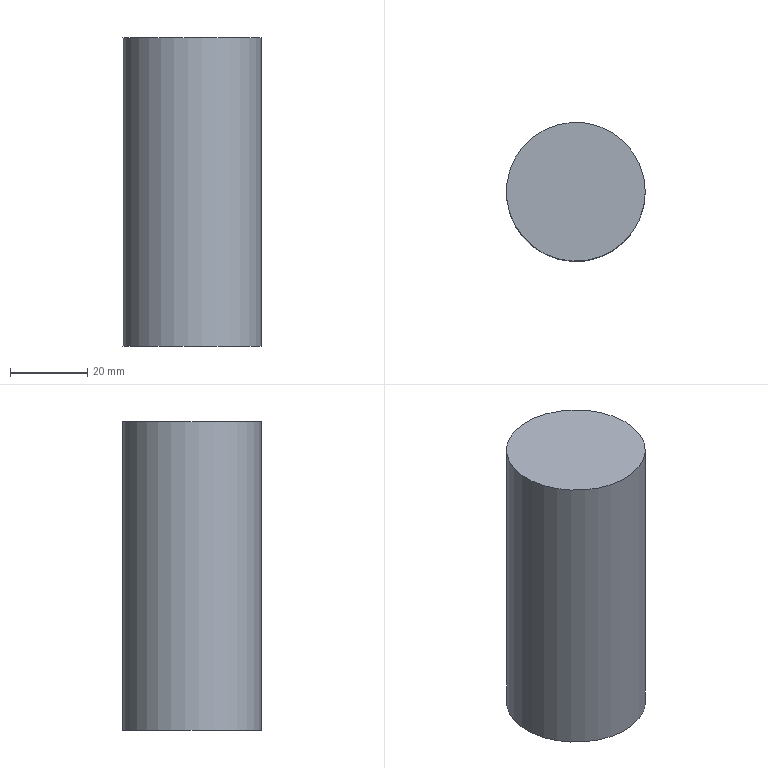Part | NX | features solid 2 | 1 solid | 3 faces | box 36 x 36 x 80 mm | volume 81430 mm3 | plane 2 | cylinder 1 | commonest cylinder face diameters 36 x1
STEP:
#1=CARTESIAN_POINT('',(-652.,375.,120.));
#2=VERTEX_POINT('',#1);
#3=CARTESIAN_POINT('',(-670.,375.,120.));
#4=DIRECTION('',(0.,0.,1.));
#5=DIRECTION('',(1.,0.,0.));
#6=AXIS2_PLACEMENT_3D('',#3,#4,#5);
#7=CIRCLE('',#6,18.);
#8=EDGE_CURVE('',#2,#2,#7,.T.);
#9=ORIENTED_EDGE('',*,*,#8,.T.);
#10=EDGE_LOOP('',(#9));
#11=FACE_BOUND('',#10,.T.);
#12=CARTESIAN_POINT('',(-652.,375.,200.));
#13=VERTEX_POINT('',#12);
#14=CARTESIAN_POINT('',(-670.,375.,200.));
#15=DIRECTION('',(0.,0.,1.));
#16=DIRECTION('',(1.,0.,0.));
#17=AXIS2_PLACEMENT_3D('',#14,#15,#16);
#18=CIRCLE('',#17,18.);
#19=EDGE_CURVE('',#13,#13,#18,.T.);
#20=ORIENTED_EDGE('',*,*,#19,.F.);
#21=EDGE_LOOP('',(#20));
#22=FACE_BOUND('',#21,.T.);
#23=CARTESIAN_POINT('',(-670.,375.,120.));
#24=DIRECTION('',(0.,0.,1.));
#25=DIRECTION('',(-1.,0.,0.));
#26=AXIS2_PLACEMENT_3D('',#23,#24,#25);
#27=CYLINDRICAL_SURFACE('',#26,18.);
#28=ADVANCED_FACE('',(#11,#22),#27,.T.);
#29=ORIENTED_EDGE('',*,*,#8,.F.);
#30=EDGE_LOOP('',(#29));
#31=FACE_BOUND('',#30,.T.);
#32=CARTESIAN_POINT('',(-670.,375.,120.));
#33=DIRECTION('',(0.,0.,-1.));
#34=DIRECTION('',(1.,0.,0.));
#35=AXIS2_PLACEMENT_3D('',#32,#33,#34);
#36=PLANE('',#35);
#37=ADVANCED_FACE('',(#31),#36,.T.);
#38=ORIENTED_EDGE('',*,*,#19,.T.);
#39=EDGE_LOOP('',(#38));
#40=FACE_BOUND('',#39,.T.);
#41=CARTESIAN_POINT('',(-670.,375.,200.));
#42=DIRECTION('',(0.,0.,-1.));
#43=DIRECTION('',(1.,0.,0.));
#44=AXIS2_PLACEMENT_3D('',#41,#42,#43);
#45=PLANE('',#44);
#46=ADVANCED_FACE('',(#40),#45,.F.);
#47=CLOSED_SHELL('',(#28,#37,#46));
#48=MANIFOLD_SOLID_BREP('',#47);
#49=(LENGTH_UNIT()NAMED_UNIT(*)SI_UNIT(.MILLI.,.METRE.));
#50=UNCERTAINTY_MEASURE_WITH_UNIT(LENGTH_MEASURE(0.00001),#49,'','');
#51=(NAMED_UNIT(*)PLANE_ANGLE_UNIT()SI_UNIT($,.RADIAN.));
#52=(NAMED_UNIT(*)SI_UNIT($,.STERADIAN.)SOLID_ANGLE_UNIT());
#53=(GEOMETRIC_REPRESENTATION_CONTEXT(3)GLOBAL_UNCERTAINTY_ASSIGNED_CONTEXT((#50))GLOBAL_UNIT_ASSIGNED_CONTEXT((#49,#51,#52))REPRESENTATION_CONTEXT('',''));
#54=ADVANCED_BREP_SHAPE_REPRESENTATION('',(#48),#53);